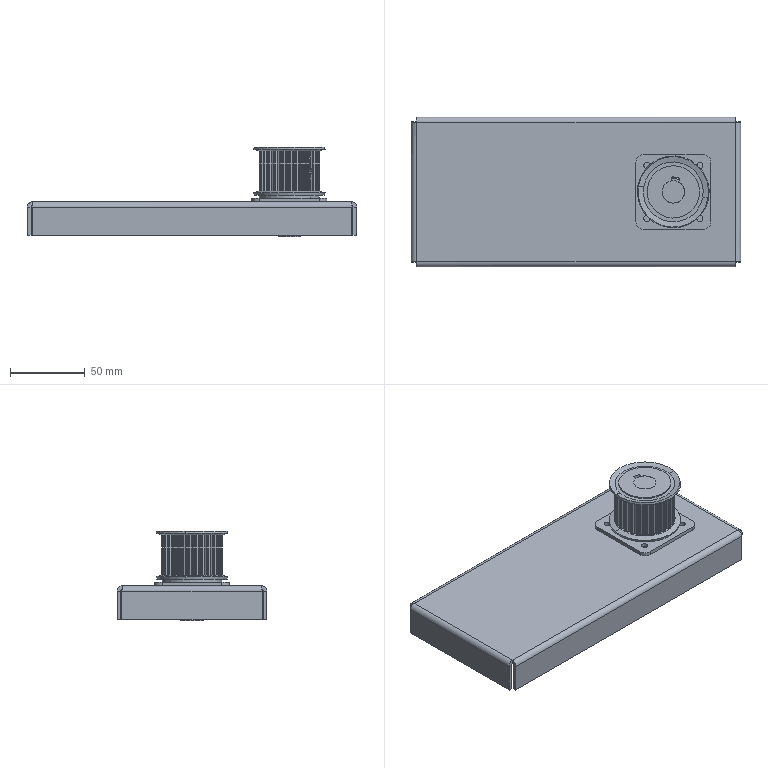Part | SolidWorks | 18 solids | 629 faces | box 220 x 100 x 60.061 mm | volume 148647 mm3 | cylinder 351 | plane 132 | sphere 84 | torus 34 | cone 20 | spline 8 | commonest cylinder face diameters 0.5 x56 6.55 x56 1.1 x52 36.88 x28 40.42 x27 22.95 x21